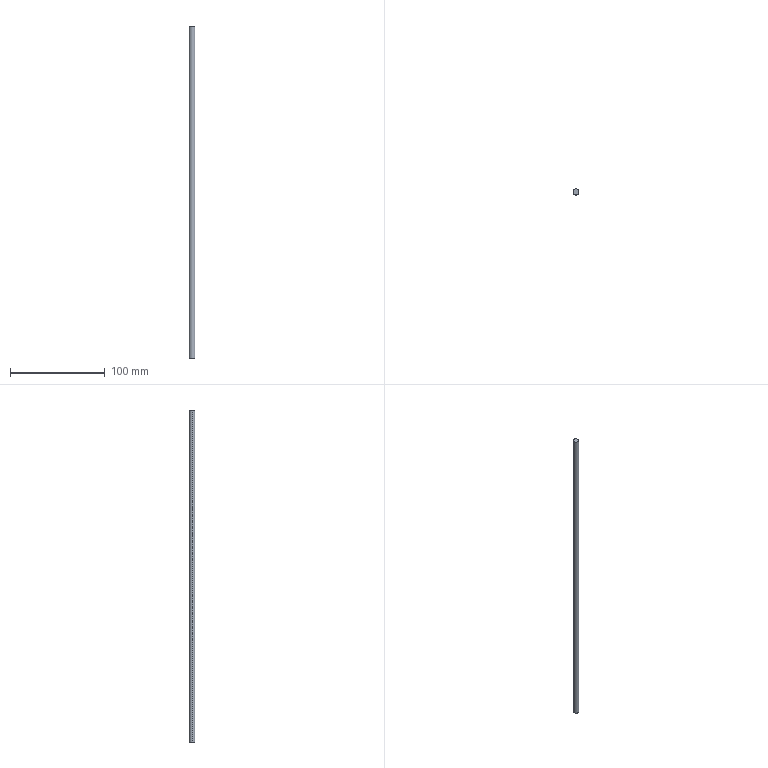Part | SolidWorks | features Extrusion 1 | 1 solid | 4 faces | box 6 x 6 x 350 mm | volume 9896 mm3 | cylinder 2 | plane 2 | commonest cylinder face diameters 6 x2
STEP:
#1=CARTESIAN_POINT('',(3.,0.,350.));
#2=VERTEX_POINT('',#1);
#3=CARTESIAN_POINT('',(-3.,0.,350.));
#4=VERTEX_POINT('',#3);
#5=CARTESIAN_POINT('',(0.,0.,350.));
#6=DIRECTION('',(0.,0.,1.));
#7=DIRECTION('',(1.,0.,0.));
#8=AXIS2_PLACEMENT_3D('',#5,#6,#7);
#9=CIRCLE('',#8,3.);
#10=EDGE_CURVE('',#2,#4,#9,.T.);
#11=ORIENTED_EDGE('',*,*,#10,.F.);
#12=CARTESIAN_POINT('',(3.,0.,0.));
#13=VERTEX_POINT('',#12);
#14=CARTESIAN_POINT('',(3.,0.,350.));
#15=DIRECTION('',(0.,0.,-1.));
#16=VECTOR('',#15,1000.);
#17=LINE('',#14,#16);
#18=EDGE_CURVE('',#2,#13,#17,.T.);
#19=ORIENTED_EDGE('',*,*,#18,.T.);
#20=CARTESIAN_POINT('',(-3.,0.,0.));
#21=VERTEX_POINT('',#20);
#22=CARTESIAN_POINT('',(0.,0.,0.));
#23=DIRECTION('',(0.,0.,1.));
#24=DIRECTION('',(1.,0.,0.));
#25=AXIS2_PLACEMENT_3D('',#22,#23,#24);
#26=CIRCLE('',#25,3.);
#27=EDGE_CURVE('',#13,#21,#26,.T.);
#28=ORIENTED_EDGE('',*,*,#27,.T.);
#29=CARTESIAN_POINT('',(-3.,0.,350.));
#30=DIRECTION('',(0.,0.,-1.));
#31=VECTOR('',#30,1000.);
#32=LINE('',#29,#31);
#33=EDGE_CURVE('',#4,#21,#32,.T.);
#34=ORIENTED_EDGE('',*,*,#33,.F.);
#35=EDGE_LOOP('',(#11,#19,#28,#34));
#36=FACE_OUTER_BOUND('',#35,.T.);
#37=CARTESIAN_POINT('',(0.,0.,350.));
#38=DIRECTION('',(0.,0.,-1.));
#39=DIRECTION('',(-1.,0.,0.));
#40=AXIS2_PLACEMENT_3D('',#37,#38,#39);
#41=CYLINDRICAL_SURFACE('',#40,3.);
#42=ADVANCED_FACE('',(#36),#41,.T.);
#43=ORIENTED_EDGE('',*,*,#18,.F.);
#44=CARTESIAN_POINT('',(0.,0.,350.));
#45=DIRECTION('',(0.,0.,1.));
#46=DIRECTION('',(1.,0.,0.));
#47=AXIS2_PLACEMENT_3D('',#44,#45,#46);
#48=CIRCLE('',#47,3.);
#49=EDGE_CURVE('',#4,#2,#48,.T.);
#50=ORIENTED_EDGE('',*,*,#49,.F.);
#51=ORIENTED_EDGE('',*,*,#33,.T.);
#52=CARTESIAN_POINT('',(0.,0.,0.));
#53=DIRECTION('',(0.,0.,1.));
#54=DIRECTION('',(1.,0.,0.));
#55=AXIS2_PLACEMENT_3D('',#52,#53,#54);
#56=CIRCLE('',#55,3.);
#57=EDGE_CURVE('',#21,#13,#56,.T.);
#58=ORIENTED_EDGE('',*,*,#57,.T.);
#59=EDGE_LOOP('',(#43,#50,#51,#58));
#60=FACE_OUTER_BOUND('',#59,.T.);
#61=CARTESIAN_POINT('',(0.,0.,350.));
#62=DIRECTION('',(0.,0.,-1.));
#63=DIRECTION('',(-1.,0.,0.));
#64=AXIS2_PLACEMENT_3D('',#61,#62,#63);
#65=CYLINDRICAL_SURFACE('',#64,3.);
#66=ADVANCED_FACE('',(#60),#65,.T.);
#67=ORIENTED_EDGE('',*,*,#49,.T.);
#68=ORIENTED_EDGE('',*,*,#10,.T.);
#69=EDGE_LOOP('',(#67,#68));
#70=FACE_OUTER_BOUND('',#69,.T.);
#71=CARTESIAN_POINT('',(0.,0.,350.));
#72=DIRECTION('',(0.,0.,1.));
#73=DIRECTION('',(1.,0.,0.));
#74=AXIS2_PLACEMENT_3D('',#71,#72,#73);
#75=PLANE('',#74);
#76=ADVANCED_FACE('',(#70),#75,.T.);
#77=ORIENTED_EDGE('',*,*,#57,.F.);
#78=ORIENTED_EDGE('',*,*,#27,.F.);
#79=EDGE_LOOP('',(#77,#78));
#80=FACE_OUTER_BOUND('',#79,.T.);
#81=CARTESIAN_POINT('',(0.,0.,0.));
#82=DIRECTION('',(0.,0.,1.));
#83=DIRECTION('',(1.,0.,0.));
#84=AXIS2_PLACEMENT_3D('',#81,#82,#83);
#85=PLANE('',#84);
#86=ADVANCED_FACE('',(#80),#85,.F.);
#87=CLOSED_SHELL('',(#42,#66,#76,#86));
#88=MANIFOLD_SOLID_BREP('',#87);
#89=CARTESIAN_POINT('',(0.,0.,0.));
#90=DIRECTION('',(0.,0.,1.));
#91=DIRECTION('',(1.,0.,0.));
#92=AXIS2_PLACEMENT_3D('',#89,#90,#91);
#93=(LENGTH_UNIT()NAMED_UNIT(*)SI_UNIT(.MILLI.,.METRE.));
#94=UNCERTAINTY_MEASURE_WITH_UNIT(LENGTH_MEASURE(0.00001),#93,'','');
#95=(NAMED_UNIT(*)PLANE_ANGLE_UNIT()SI_UNIT($,.RADIAN.));
#96=(NAMED_UNIT(*)SI_UNIT($,.STERADIAN.)SOLID_ANGLE_UNIT());
#97=(GEOMETRIC_REPRESENTATION_CONTEXT(3)GLOBAL_UNCERTAINTY_ASSIGNED_CONTEXT((#94))GLOBAL_UNIT_ASSIGNED_CONTEXT((#93,#95,#96))REPRESENTATION_CONTEXT('',''));
#98=ADVANCED_BREP_SHAPE_REPRESENTATION('',(#88,#92),#97);